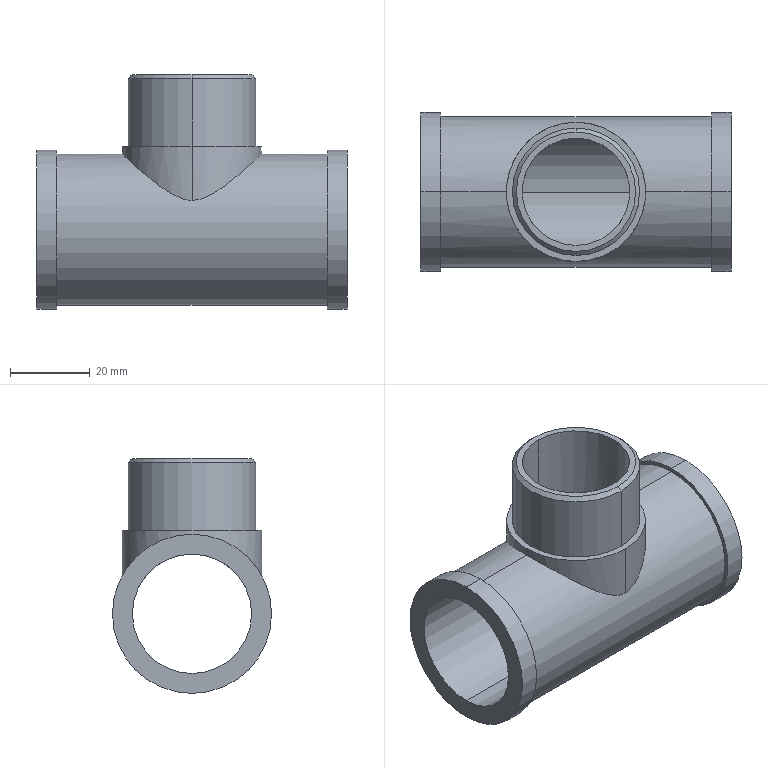Part | SolidWorks | features ICE 2, Revolution 2, Chamfer 1 | 1 solid | 22 faces | box 78 x 40 x 59 mm | volume 38405 mm3 | cylinder 14 | plane 6 | cone 2 | commonest cylinder face diameters 40 x4 27 x2 30 x2 32 x2 35 x2 38 x2
STEP:
#1=CARTESIAN_POINT('',(39.,-15.,39.));
#2=VERTEX_POINT('',#1);
#3=CARTESIAN_POINT('',(39.,15.,39.));
#4=VERTEX_POINT('',#3);
#5=CARTESIAN_POINT('',(39.,0.,39.));
#6=DIRECTION('',(0.,0.,1.));
#7=DIRECTION('',(0.,1.,0.));
#8=AXIS2_PLACEMENT_3D('',#5,#6,#7);
#9=CIRCLE('',#8,15.);
#10=EDGE_CURVE('',#2,#4,#9,.T.);
#11=ORIENTED_EDGE('',*,*,#10,.F.);
#12=CARTESIAN_POINT('',(39.,-16.,38.));
#13=VERTEX_POINT('',#12);
#14=CARTESIAN_POINT('',(39.,-16.,38.));
#15=DIRECTION('',(0.,-0.7071,-0.7071));
#16=VECTOR('',#15,1000.);
#17=LINE('',#14,#16);
#18=EDGE_CURVE('',#2,#13,#17,.T.);
#19=ORIENTED_EDGE('',*,*,#18,.T.);
#20=CARTESIAN_POINT('',(39.,16.,38.));
#21=VERTEX_POINT('',#20);
#22=CARTESIAN_POINT('',(39.,0.,38.));
#23=DIRECTION('',(0.,0.,-1.));
#24=DIRECTION('',(0.,1.,0.));
#25=AXIS2_PLACEMENT_3D('',#22,#23,#24);
#26=CIRCLE('',#25,16.);
#27=EDGE_CURVE('',#21,#13,#26,.T.);
#28=ORIENTED_EDGE('',*,*,#27,.F.);
#29=CARTESIAN_POINT('',(39.,16.,38.));
#30=DIRECTION('',(0.,0.7071,-0.7071));
#31=VECTOR('',#30,1000.);
#32=LINE('',#29,#31);
#33=EDGE_CURVE('',#4,#21,#32,.T.);
#34=ORIENTED_EDGE('',*,*,#33,.F.);
#35=EDGE_LOOP('',(#11,#19,#28,#34));
#36=FACE_OUTER_BOUND('',#35,.T.);
#37=CARTESIAN_POINT('',(39.,0.,38.));
#38=DIRECTION('',(0.,0.,-1.));
#39=DIRECTION('',(0.,1.,0.));
#40=AXIS2_PLACEMENT_3D('',#37,#38,#39);
#41=CONICAL_SURFACE('',#40,16.,0.7854);
#42=ADVANCED_FACE('',(#36),#41,.T.);
#43=CARTESIAN_POINT('',(78.,0.,-15.));
#44=VERTEX_POINT('',#43);
#45=CARTESIAN_POINT('',(78.,0.,15.));
#46=VERTEX_POINT('',#45);
#47=CARTESIAN_POINT('',(78.,0.,0.));
#48=DIRECTION('',(-1.,0.,0.));
#49=DIRECTION('',(0.,0.,1.));
#50=AXIS2_PLACEMENT_3D('',#47,#48,#49);
#51=CIRCLE('',#50,15.);
#52=EDGE_CURVE('',#44,#46,#51,.T.);
#53=ORIENTED_EDGE('',*,*,#52,.F.);
#54=CARTESIAN_POINT('',(0.,0.,-15.));
#55=VERTEX_POINT('',#54);
#56=CARTESIAN_POINT('',(0.,0.,-15.));
#57=DIRECTION('',(-1.,0.,0.));
#58=VECTOR('',#57,1000.);
#59=LINE('',#56,#58);
#60=EDGE_CURVE('',#44,#55,#59,.T.);
#61=ORIENTED_EDGE('',*,*,#60,.T.);
#62=CARTESIAN_POINT('',(0.,0.,15.));
#63=VERTEX_POINT('',#62);
#64=CARTESIAN_POINT('',(0.,0.,0.));
#65=DIRECTION('',(-1.,0.,0.));
#66=DIRECTION('',(0.,0.,1.));
#67=AXIS2_PLACEMENT_3D('',#64,#65,#66);
#68=CIRCLE('',#67,15.);
#69=EDGE_CURVE('',#55,#63,#68,.T.);
#70=ORIENTED_EDGE('',*,*,#69,.T.);
#71=CARTESIAN_POINT('',(25.5,0.,15.));
#72=VERTEX_POINT('',#71);
#73=CARTESIAN_POINT('',(0.,0.,15.));
#74=DIRECTION('',(-1.,0.,0.));
#75=VECTOR('',#74,1000.);
#76=LINE('',#73,#75);
#77=EDGE_CURVE('',#72,#63,#76,.T.);
#78=ORIENTED_EDGE('',*,*,#77,.F.);
#79=CARTESIAN_POINT('',(39.,-13.5,6.538));
#80=VERTEX_POINT('',#79);
#81=CARTESIAN_POINT('',(39.,-13.5,6.538));
#82=CARTESIAN_POINT('',(38.513,-13.5,6.538));
#83=CARTESIAN_POINT('',(38.035,-13.474,6.593));
#84=CARTESIAN_POINT('',(37.329,-13.398,6.745));
#85=CARTESIAN_POINT('',(37.094,-13.367,6.807));
#86=CARTESIAN_POINT('',(36.634,-13.293,6.95));
#87=CARTESIAN_POINT('',(36.41,-13.251,7.03));
#88=CARTESIAN_POINT('',(35.749,-13.11,7.291));
#89=CARTESIAN_POINT('',(35.325,-12.997,7.492));
#90=CARTESIAN_POINT('',(34.503,-12.736,7.928));
#91=CARTESIAN_POINT('',(34.103,-12.587,8.164));
#92=CARTESIAN_POINT('',(32.947,-12.096,8.89));
#93=CARTESIAN_POINT('',(32.232,-11.709,9.4));
#94=CARTESIAN_POINT('',(31.215,-11.037,10.164));
#95=CARTESIAN_POINT('',(30.885,-10.797,10.419));
#96=CARTESIAN_POINT('',(30.244,-10.284,10.926));
#97=CARTESIAN_POINT('',(29.931,-10.009,11.179));
#98=CARTESIAN_POINT('',(29.032,-9.142,11.916));
#99=CARTESIAN_POINT('',(28.482,-8.507,12.382));
#100=CARTESIAN_POINT('',(27.736,-7.454,13.024));
#101=CARTESIAN_POINT('',(27.5,-7.086,13.228));
#102=CARTESIAN_POINT('',(27.058,-6.312,13.614));
#103=CARTESIAN_POINT('',(26.853,-5.909,13.794));
#104=CARTESIAN_POINT('',(26.484,-5.081,14.12));
#105=CARTESIAN_POINT('',(26.319,-4.654,14.267));
#106=CARTESIAN_POINT('',(26.102,-3.992,14.461));
#107=CARTESIAN_POINT('',(26.034,-3.768,14.521));
#108=CARTESIAN_POINT('',(25.911,-3.313,14.632));
#109=CARTESIAN_POINT('',(25.854,-3.08,14.682));
#110=CARTESIAN_POINT('',(25.602,-1.914,14.908));
#111=CARTESIAN_POINT('',(25.5,-0.9652,15.));
#112=CARTESIAN_POINT('',(25.5,0.,15.));
#113=B_SPLINE_CURVE_WITH_KNOTS('',3,(#81,#82,#83,#84,#85,#86,#87,#88,#89,#90,#91,#92,#93,#94,#95,#96,#97,#98,#99,#100,#101,#102,#103,#104,#105,#106,#107,#108,#109,#110,#111,#112),.UNSPECIFIED.,.F.,.F.,(4,2,2,2,2,2,2,2,2,2,2,2,2,2,2,4),(0.02301,0.02446,0.02518,0.0259,0.02734,0.02879,0.03167,0.03311,0.03456,0.03744,0.03889,0.04033,0.04177,0.04249,0.04321,0.0461),.UNSPECIFIED.);
#114=EDGE_CURVE('',#80,#72,#113,.T.);
#115=ORIENTED_EDGE('',*,*,#114,.F.);
#116=CARTESIAN_POINT('',(52.5,0.,15.));
#117=VERTEX_POINT('',#116);
#118=CARTESIAN_POINT('',(52.5,0.,15.));
#119=CARTESIAN_POINT('',(52.5,-0.9754,15.));
#120=CARTESIAN_POINT('',(52.396,-1.925,14.906));
#121=CARTESIAN_POINT('',(52.096,-3.313,14.637));
#122=CARTESIAN_POINT('',(51.971,-3.773,14.525));
#123=CARTESIAN_POINT('',(51.679,-4.658,14.266));
#124=CARTESIAN_POINT('',(51.514,-5.086,14.119));
#125=CARTESIAN_POINT('',(51.145,-5.913,13.793));
#126=CARTESIAN_POINT('',(50.942,-6.312,13.614));
#127=CARTESIAN_POINT('',(50.5,-7.085,13.228));
#128=CARTESIAN_POINT('',(50.263,-7.456,13.022));
#129=CARTESIAN_POINT('',(49.515,-8.51,12.38));
#130=CARTESIAN_POINT('',(48.967,-9.143,11.915));
#131=CARTESIAN_POINT('',(48.072,-10.006,11.181));
#132=CARTESIAN_POINT('',(47.76,-10.28,10.929));
#133=CARTESIAN_POINT('',(47.117,-10.795,10.421));
#134=CARTESIAN_POINT('',(46.787,-11.035,10.165));
#135=CARTESIAN_POINT('',(45.768,-11.71,9.399));
#136=CARTESIAN_POINT('',(45.052,-12.096,8.889));
#137=CARTESIAN_POINT('',(43.898,-12.587,8.164));
#138=CARTESIAN_POINT('',(43.498,-12.736,7.928));
#139=CARTESIAN_POINT('',(42.675,-12.997,7.492));
#140=CARTESIAN_POINT('',(42.251,-13.111,7.291));
#141=CARTESIAN_POINT('',(41.367,-13.299,6.942));
#142=CARTESIAN_POINT('',(40.906,-13.373,6.795));
#143=CARTESIAN_POINT('',(40.204,-13.448,6.644));
#144=CARTESIAN_POINT('',(39.967,-13.467,6.605));
#145=CARTESIAN_POINT('',(39.487,-13.493,6.552));
#146=CARTESIAN_POINT('',(39.243,-13.5,6.538));
#147=CARTESIAN_POINT('',(39.,-13.5,6.538));
#148=B_SPLINE_CURVE_WITH_KNOTS('',3,(#118,#119,#120,#121,#122,#123,#124,#125,#126,#127,#128,#129,#130,#131,#132,#133,#134,#135,#136,#137,#138,#139,#140,#141,#142,#143,#144,#145,#146,#147),.UNSPECIFIED.,.F.,.F.,(4,2,2,2,2,2,2,2,2,2,2,2,2,2,4),(0.,0.002877,0.004315,0.005754,0.007192,0.008631,0.01151,0.01295,0.01438,0.01726,0.0187,0.02014,0.02158,0.0223,0.02301),.UNSPECIFIED.);
#149=EDGE_CURVE('',#117,#80,#148,.T.);
#150=ORIENTED_EDGE('',*,*,#149,.F.);
#151=CARTESIAN_POINT('',(0.,0.,15.));
#152=DIRECTION('',(-1.,0.,0.));
#153=VECTOR('',#152,1000.);
#154=LINE('',#151,#153);
#155=EDGE_CURVE('',#46,#117,#154,.T.);
#156=ORIENTED_EDGE('',*,*,#155,.F.);
#157=EDGE_LOOP('',(#53,#61,#70,#78,#115,#150,#156));
#158=FACE_OUTER_BOUND('',#157,.T.);
#159=CARTESIAN_POINT('',(0.,0.,0.));
#160=DIRECTION('',(-1.,0.,0.));
#161=DIRECTION('',(0.,0.,1.));
#162=AXIS2_PLACEMENT_3D('',#159,#160,#161);
#163=CYLINDRICAL_SURFACE('',#162,15.);
#164=ADVANCED_FACE('',(#158),#163,.F.);
#165=CARTESIAN_POINT('',(39.,17.5,21.));
#166=VERTEX_POINT('',#165);
#167=CARTESIAN_POINT('',(39.,-17.5,21.));
#168=VERTEX_POINT('',#167);
#169=CARTESIAN_POINT('',(39.,0.,21.));
#170=DIRECTION('',(0.,0.,-1.));
#171=DIRECTION('',(0.,1.,0.));
#172=AXIS2_PLACEMENT_3D('',#169,#170,#171);
#173=CIRCLE('',#172,17.5);
#174=EDGE_CURVE('',#166,#168,#173,.T.);
#175=ORIENTED_EDGE('',*,*,#174,.T.);
#176=CARTESIAN_POINT('',(39.,-17.5,7.399));
#177=VERTEX_POINT('',#176);
#178=CARTESIAN_POINT('',(39.,-17.5,0.));
#179=DIRECTION('',(0.,0.,-1.));
#180=VECTOR('',#179,1000.);
#181=LINE('',#178,#180);
#182=EDGE_CURVE('',#168,#177,#181,.T.);
#183=ORIENTED_EDGE('',*,*,#182,.T.);
#184=CARTESIAN_POINT('',(56.5,0.,19.));
#185=VERTEX_POINT('',#184);
#186=CARTESIAN_POINT('',(39.,-17.5,7.399));
#187=CARTESIAN_POINT('',(39.315,-17.5,7.399));
#188=CARTESIAN_POINT('',(39.63,-17.491,7.42));
#189=CARTESIAN_POINT('',(40.259,-17.457,7.499));
#190=CARTESIAN_POINT('',(40.574,-17.432,7.559));
#191=CARTESIAN_POINT('',(41.493,-17.333,7.785));
#192=CARTESIAN_POINT('',(42.078,-17.237,7.998));
#193=CARTESIAN_POINT('',(42.93,-17.055,8.375));
#194=CARTESIAN_POINT('',(43.211,-16.988,8.51));
#195=CARTESIAN_POINT('',(43.76,-16.843,8.795));
#196=CARTESIAN_POINT('',(44.028,-16.764,8.943));
#197=CARTESIAN_POINT('',(44.817,-16.514,9.402));
#198=CARTESIAN_POINT('',(45.322,-16.327,9.726));
#199=CARTESIAN_POINT('',(46.304,-15.912,10.391));
#200=CARTESIAN_POINT('',(46.781,-15.684,10.733));
#201=CARTESIAN_POINT('',(47.711,-15.187,11.425));
#202=CARTESIAN_POINT('',(48.166,-14.917,11.777));
#203=CARTESIAN_POINT('',(49.486,-14.05,12.823));
#204=CARTESIAN_POINT('',(50.31,-13.397,13.51));
#205=CARTESIAN_POINT('',(51.47,-12.29,14.499));
#206=CARTESIAN_POINT('',(51.843,-11.899,14.821));
#207=CARTESIAN_POINT('',(52.564,-11.071,15.45));
#208=CARTESIAN_POINT('',(52.91,-10.633,15.755));
#209=CARTESIAN_POINT('',(53.887,-9.267,16.622));
#210=CARTESIAN_POINT('',(54.463,-8.279,17.141));
#211=CARTESIAN_POINT('',(55.073,-6.928,17.694));
#212=CARTESIAN_POINT('',(55.19,-6.651,17.8));
#213=CARTESIAN_POINT('',(55.409,-6.09,18.));
#214=CARTESIAN_POINT('',(55.511,-5.807,18.093));
#215=CARTESIAN_POINT('',(55.798,-4.945,18.355));
#216=CARTESIAN_POINT('',(55.96,-4.357,18.504));
#217=CARTESIAN_POINT('',(56.159,-3.452,18.686));
#218=CARTESIAN_POINT('',(56.218,-3.147,18.74));
#219=CARTESIAN_POINT('',(56.319,-2.529,18.834));
#220=CARTESIAN_POINT('',(56.362,-2.215,18.873));
#221=CARTESIAN_POINT('',(56.431,-1.585,18.936));
#222=CARTESIAN_POINT('',(56.457,-1.27,18.96));
#223=CARTESIAN_POINT('',(56.491,-0.6365,18.992));
#224=CARTESIAN_POINT('',(56.5,-0.3201,19.));
#225=CARTESIAN_POINT('',(56.5,0.,19.));
#226=B_SPLINE_CURVE_WITH_KNOTS('',3,(#186,#187,#188,#189,#190,#191,#192,#193,#194,#195,#196,#197,#198,#199,#200,#201,#202,#203,#204,#205,#206,#207,#208,#209,#210,#211,#212,#213,#214,#215,#216,#217,#218,#219,#220,#221,#222,#223,#224,#225),.UNSPECIFIED.,.F.,.F.,(4,2,2,2,2,2,2,2,2,2,2,2,2,2,2,2,2,2,2,4),(0.09049,0.09144,0.09238,0.09427,0.09521,0.09616,0.09805,0.09993,0.1018,0.1056,0.1075,0.1094,0.1132,0.1141,0.115,0.1169,0.1179,0.1188,0.1198,0.1207),.UNSPECIFIED.);
#227=EDGE_CURVE('',#177,#185,#226,.T.);
#228=ORIENTED_EDGE('',*,*,#227,.T.);
#229=CARTESIAN_POINT('',(39.,17.5,7.399));
#230=VERTEX_POINT('',#229);
#231=CARTESIAN_POINT('',(56.5,0.,19.));
#232=CARTESIAN_POINT('',(56.5,1.276,19.));
#233=CARTESIAN_POINT('',(56.362,2.518,18.873));
#234=CARTESIAN_POINT('',(55.967,4.332,18.51));
#235=CARTESIAN_POINT('',(55.801,4.933,18.358));
#236=CARTESIAN_POINT('',(55.419,6.087,18.009));
#237=CARTESIAN_POINT('',(55.201,6.643,17.81));
#238=CARTESIAN_POINT('',(54.716,7.72,17.371));
#239=CARTESIAN_POINT('',(54.45,8.239,17.13));
#240=CARTESIAN_POINT('',(53.871,9.244,16.609));
#241=CARTESIAN_POINT('',(53.561,9.723,16.333));
#242=CARTESIAN_POINT('',(52.586,11.087,15.468));
#243=CARTESIAN_POINT('',(51.871,11.905,14.841));
#244=CARTESIAN_POINT('',(50.708,13.018,13.849));
#245=CARTESIAN_POINT('',(50.303,13.37,13.508));
#246=CARTESIAN_POINT('',(49.472,14.031,12.82));
#247=CARTESIAN_POINT('',(49.046,14.339,12.474));
#248=CARTESIAN_POINT('',(47.731,15.203,11.432));
#249=CARTESIAN_POINT('',(46.809,15.698,10.733));
#250=CARTESIAN_POINT('',(45.326,16.325,9.728));
#251=CARTESIAN_POINT('',(44.814,16.515,9.401));
#252=CARTESIAN_POINT('',(43.76,16.849,8.788));
#253=CARTESIAN_POINT('',(43.215,16.995,8.5));
#254=CARTESIAN_POINT('',(42.074,17.238,7.996));
#255=CARTESIAN_POINT('',(41.485,17.333,7.783));
#256=CARTESIAN_POINT('',(40.573,17.432,7.559));
#257=CARTESIAN_POINT('',(40.263,17.457,7.5));
#258=CARTESIAN_POINT('',(39.632,17.491,7.42));
#259=CARTESIAN_POINT('',(39.314,17.5,7.399));
#260=CARTESIAN_POINT('',(39.,17.5,7.399));
#261=B_SPLINE_CURVE_WITH_KNOTS('',3,(#231,#232,#233,#234,#235,#236,#237,#238,#239,#240,#241,#242,#243,#244,#245,#246,#247,#248,#249,#250,#251,#252,#253,#254,#255,#256,#257,#258,#259,#260),.UNSPECIFIED.,.F.,.F.,(4,2,2,2,2,2,2,2,2,2,2,2,2,2,4),(0.,0.003764,0.005646,0.007528,0.00941,0.01129,0.01506,0.01694,0.01882,0.02258,0.02447,0.02635,0.02823,0.02917,0.03011),.UNSPECIFIED.);
#262=EDGE_CURVE('',#185,#230,#261,.T.);
#263=ORIENTED_EDGE('',*,*,#262,.T.);
#264=CARTESIAN_POINT('',(39.,17.5,0.));
#265=DIRECTION('',(0.,0.,-1.));
#266=VECTOR('',#265,1000.);
#267=LINE('',#264,#266);
#268=EDGE_CURVE('',#166,#230,#267,.T.);
#269=ORIENTED_EDGE('',*,*,#268,.F.);
#270=EDGE_LOOP('',(#175,#183,#228,#263,#269));
#271=FACE_OUTER_BOUND('',#270,.T.);
#272=CARTESIAN_POINT('',(39.,0.,0.));
#273=DIRECTION('',(0.,0.,-1.));
#274=DIRECTION('',(0.,1.,0.));
#275=AXIS2_PLACEMENT_3D('',#272,#273,#274);
#276=CYLINDRICAL_SURFACE('',#275,17.5);
#277=ADVANCED_FACE('',(#271),#276,.T.);
#278=CARTESIAN_POINT('',(39.,-13.5,39.));
#279=VERTEX_POINT('',#278);
#280=CARTESIAN_POINT('',(39.,13.5,39.));
#281=VERTEX_POINT('',#280);
#282=CARTESIAN_POINT('',(39.,0.,39.));
#283=DIRECTION('',(0.,0.,-1.));
#284=DIRECTION('',(0.,1.,0.));
#285=AXIS2_PLACEMENT_3D('',#282,#283,#284);
#286=CIRCLE('',#285,13.5);
#287=EDGE_CURVE('',#279,#281,#286,.T.);
#288=ORIENTED_EDGE('',*,*,#287,.F.);
#289=CARTESIAN_POINT('',(39.,-13.5,0.));
#290=DIRECTION('',(0.,0.,-1.));
#291=VECTOR('',#290,1000.);
#292=LINE('',#289,#291);
#293=EDGE_CURVE('',#279,#80,#292,.T.);
#294=ORIENTED_EDGE('',*,*,#293,.T.);
#295=ORIENTED_EDGE('',*,*,#114,.T.);
#296=CARTESIAN_POINT('',(39.,13.5,6.538));
#297=VERTEX_POINT('',#296);
#298=CARTESIAN_POINT('',(25.5,0.,15.));
#299=CARTESIAN_POINT('',(25.5,0.4816,15.));
#300=CARTESIAN_POINT('',(25.526,0.9708,14.976));
#301=CARTESIAN_POINT('',(25.63,1.926,14.884));
#302=CARTESIAN_POINT('',(25.706,2.396,14.815));
#303=CARTESIAN_POINT('',(25.906,3.32,14.636));
#304=CARTESIAN_POINT('',(26.03,3.775,14.525));
#305=CARTESIAN_POINT('',(26.323,4.665,14.264));
#306=CARTESIAN_POINT('',(26.489,5.093,14.116));
#307=CARTESIAN_POINT('',(26.859,5.92,13.789));
#308=CARTESIAN_POINT('',(27.062,6.319,13.611));
#309=CARTESIAN_POINT('',(27.503,7.09,13.225));
#310=CARTESIAN_POINT('',(27.741,7.462,13.019));
#311=CARTESIAN_POINT('',(28.49,8.517,12.375));
#312=CARTESIAN_POINT('',(29.039,9.149,11.91));
#313=CARTESIAN_POINT('',(30.231,10.297,10.933));
#314=CARTESIAN_POINT('',(30.877,10.814,10.417));
#315=CARTESIAN_POINT('',(32.237,11.712,9.396));
#316=CARTESIAN_POINT('',(32.952,12.098,8.886));
#317=CARTESIAN_POINT('',(34.103,12.588,8.163));
#318=CARTESIAN_POINT('',(34.502,12.736,7.928));
#319=CARTESIAN_POINT('',(35.327,12.998,7.491));
#320=CARTESIAN_POINT('',(35.751,13.111,7.29));
#321=CARTESIAN_POINT('',(36.633,13.299,6.942));
#322=CARTESIAN_POINT('',(37.096,13.373,6.795));
#323=CARTESIAN_POINT('',(38.034,13.474,6.593));
#324=CARTESIAN_POINT('',(38.512,13.5,6.538));
#325=CARTESIAN_POINT('',(39.,13.5,6.538));
#326=B_SPLINE_CURVE_WITH_KNOTS('',3,(#298,#299,#300,#301,#302,#303,#304,#305,#306,#307,#308,#309,#310,#311,#312,#313,#314,#315,#316,#317,#318,#319,#320,#321,#322,#323,#324,#325),.UNSPECIFIED.,.F.,.F.,(4,2,2,2,2,2,2,2,2,2,2,2,2,4),(0.0461,0.04754,0.04898,0.05042,0.05186,0.0533,0.05474,0.05762,0.0605,0.06338,0.06482,0.06626,0.0677,0.06914),.UNSPECIFIED.);
#327=EDGE_CURVE('',#72,#297,#326,.T.);
#328=ORIENTED_EDGE('',*,*,#327,.T.);
#329=CARTESIAN_POINT('',(39.,13.5,0.));
#330=DIRECTION('',(0.,0.,-1.));
#331=VECTOR('',#330,1000.);
#332=LINE('',#329,#331);
#333=EDGE_CURVE('',#281,#297,#332,.T.);
#334=ORIENTED_EDGE('',*,*,#333,.F.);
#335=EDGE_LOOP('',(#288,#294,#295,#328,#334));
#336=FACE_OUTER_BOUND('',#335,.T.);
#337=CARTESIAN_POINT('',(39.,0.,0.));
#338=DIRECTION('',(0.,0.,-1.));
#339=DIRECTION('',(0.,1.,0.));
#340=AXIS2_PLACEMENT_3D('',#337,#338,#339);
#341=CYLINDRICAL_SURFACE('',#340,13.5);
#342=ADVANCED_FACE('',(#336),#341,.F.);
#343=ORIENTED_EDGE('',*,*,#27,.T.);
#344=CARTESIAN_POINT('',(39.,-16.,21.));
#345=VERTEX_POINT('',#344);
#346=CARTESIAN_POINT('',(39.,-16.,0.));
#347=DIRECTION('',(0.,0.,-1.));
#348=VECTOR('',#347,1000.);
#349=LINE('',#346,#348);
#350=EDGE_CURVE('',#13,#345,#349,.T.);
#351=ORIENTED_EDGE('',*,*,#350,.T.);
#352=CARTESIAN_POINT('',(39.,16.,21.));
#353=VERTEX_POINT('',#352);
#354=CARTESIAN_POINT('',(39.,0.,21.));
#355=DIRECTION('',(0.,0.,-1.));
#356=DIRECTION('',(0.,1.,0.));
#357=AXIS2_PLACEMENT_3D('',#354,#355,#356);
#358=CIRCLE('',#357,16.);
#359=EDGE_CURVE('',#353,#345,#358,.T.);
#360=ORIENTED_EDGE('',*,*,#359,.F.);
#361=CARTESIAN_POINT('',(39.,16.,0.));
#362=DIRECTION('',(0.,0.,-1.));
#363=VECTOR('',#362,1000.);
#364=LINE('',#361,#363);
#365=EDGE_CURVE('',#21,#353,#364,.T.);
#366=ORIENTED_EDGE('',*,*,#365,.F.);
#367=EDGE_LOOP('',(#343,#351,#360,#366));
#368=FACE_OUTER_BOUND('',#367,.T.);
#369=CARTESIAN_POINT('',(39.,0.,0.));
#370=DIRECTION('',(0.,0.,-1.));
#371=DIRECTION('',(0.,1.,0.));
#372=AXIS2_PLACEMENT_3D('',#369,#370,#371);
#373=CYLINDRICAL_SURFACE('',#372,16.);
#374=ADVANCED_FACE('',(#368),#373,.T.);
#375=CARTESIAN_POINT('',(78.,0.,20.));
#376=VERTEX_POINT('',#375);
#377=CARTESIAN_POINT('',(78.,0.,-20.));
#378=VERTEX_POINT('',#377);
#379=CARTESIAN_POINT('',(78.,0.,0.));
#380=DIRECTION('',(-1.,0.,0.));
#381=DIRECTION('',(0.,0.,1.));
#382=AXIS2_PLACEMENT_3D('',#379,#380,#381);
#383=CIRCLE('',#382,20.);
#384=EDGE_CURVE('',#376,#378,#383,.T.);
#385=ORIENTED_EDGE('',*,*,#384,.T.);
#386=CARTESIAN_POINT('',(73.,0.,-20.));
#387=VERTEX_POINT('',#386);
#388=CARTESIAN_POINT('',(0.,0.,-20.));
#389=DIRECTION('',(-1.,0.,0.));
#390=VECTOR('',#389,1000.);
#391=LINE('',#388,#390);
#392=EDGE_CURVE('',#378,#387,#391,.T.);
#393=ORIENTED_EDGE('',*,*,#392,.T.);
#394=CARTESIAN_POINT('',(73.,0.,20.));
#395=VERTEX_POINT('',#394);
#396=CARTESIAN_POINT('',(73.,0.,0.));
#397=DIRECTION('',(-1.,0.,0.));
#398=DIRECTION('',(0.,0.,1.));
#399=AXIS2_PLACEMENT_3D('',#396,#397,#398);
#400=CIRCLE('',#399,20.);
#401=EDGE_CURVE('',#395,#387,#400,.T.);
#402=ORIENTED_EDGE('',*,*,#401,.F.);
#403=CARTESIAN_POINT('',(0.,0.,20.));
#404=DIRECTION('',(-1.,0.,0.));
#405=VECTOR('',#404,1000.);
#406=LINE('',#403,#405);
#407=EDGE_CURVE('',#376,#395,#406,.T.);
#408=ORIENTED_EDGE('',*,*,#407,.F.);
#409=EDGE_LOOP('',(#385,#393,#402,#408));
#410=FACE_OUTER_BOUND('',#409,.T.);
#411=CARTESIAN_POINT('',(0.,0.,0.));
#412=DIRECTION('',(-1.,0.,0.));
#413=DIRECTION('',(0.,0.,1.));
#414=AXIS2_PLACEMENT_3D('',#411,#412,#413);
#415=CYLINDRICAL_SURFACE('',#414,20.);
#416=ADVANCED_FACE('',(#410),#415,.T.);
#417=CARTESIAN_POINT('',(5.,0.,20.));
#418=VERTEX_POINT('',#417);
#419=CARTESIAN_POINT('',(5.,0.,-20.));
#420=VERTEX_POINT('',#419);
#421=CARTESIAN_POINT('',(5.,0.,0.));
#422=DIRECTION('',(-1.,0.,0.));
#423=DIRECTION('',(0.,0.,1.));
#424=AXIS2_PLACEMENT_3D('',#421,#422,#423);
#425=CIRCLE('',#424,20.);
#426=EDGE_CURVE('',#418,#420,#425,.T.);
#427=ORIENTED_EDGE('',*,*,#426,.T.);
#428=CARTESIAN_POINT('',(0.,0.,-20.));
#429=VERTEX_POINT('',#428);
#430=CARTESIAN_POINT('',(0.,0.,-20.));
#431=DIRECTION('',(-1.,0.,0.));
#432=VECTOR('',#431,1000.);
#433=LINE('',#430,#432);
#434=EDGE_CURVE('',#420,#429,#433,.T.);
#435=ORIENTED_EDGE('',*,*,#434,.T.);
#436=CARTESIAN_POINT('',(0.,0.,20.));
#437=VERTEX_POINT('',#436);
#438=CARTESIAN_POINT('',(0.,0.,0.));
#439=DIRECTION('',(-1.,0.,0.));
#440=DIRECTION('',(0.,0.,1.));
#441=AXIS2_PLACEMENT_3D('',#438,#439,#440);
#442=CIRCLE('',#441,20.);
#443=EDGE_CURVE('',#437,#429,#442,.T.);
#444=ORIENTED_EDGE('',*,*,#443,.F.);
#445=CARTESIAN_POINT('',(0.,0.,20.));
#446=DIRECTION('',(-1.,0.,0.));
#447=VECTOR('',#446,1000.);
#448=LINE('',#445,#447);
#449=EDGE_CURVE('',#418,#437,#448,.T.);
#450=ORIENTED_EDGE('',*,*,#449,.F.);
#451=EDGE_LOOP('',(#427,#435,#444,#450));
#452=FACE_OUTER_BOUND('',#451,.T.);
#453=CARTESIAN_POINT('',(0.,0.,0.));
#454=DIRECTION('',(-1.,0.,0.));
#455=DIRECTION('',(0.,0.,1.));
#456=AXIS2_PLACEMENT_3D('',#453,#454,#455);
#457=CYLINDRICAL_SURFACE('',#456,20.);
#458=ADVANCED_FACE('',(#452),#457,.T.);
#459=CARTESIAN_POINT('',(73.,0.,19.));
#460=VERTEX_POINT('',#459);
#461=CARTESIAN_POINT('',(73.,0.,-19.));
#462=VERTEX_POINT('',#461);
#463=CARTESIAN_POINT('',(73.,0.,0.));
#464=DIRECTION('',(-1.,0.,0.));
#465=DIRECTION('',(0.,0.,1.));
#466=AXIS2_PLACEMENT_3D('',#463,#464,#465);
#467=CIRCLE('',#466,19.);
#468=EDGE_CURVE('',#460,#462,#467,.T.);
#469=ORIENTED_EDGE('',*,*,#468,.T.);
#470=CARTESIAN_POINT('',(5.,0.,-19.));
#471=VERTEX_POINT('',#470);
#472=CARTESIAN_POINT('',(0.,0.,-19.));
#473=DIRECTION('',(-1.,0.,0.));
#474=VECTOR('',#473,1000.);
#475=LINE('',#472,#474);
#476=EDGE_CURVE('',#462,#471,#475,.T.);
#477=ORIENTED_EDGE('',*,*,#476,.T.);
#478=CARTESIAN_POINT('',(5.,0.,19.));
#479=VERTEX_POINT('',#478);
#480=CARTESIAN_POINT('',(5.,0.,0.));
#481=DIRECTION('',(-1.,0.,0.));
#482=DIRECTION('',(0.,0.,1.));
#483=AXIS2_PLACEMENT_3D('',#480,#481,#482);
#484=CIRCLE('',#483,19.);
#485=EDGE_CURVE('',#479,#471,#484,.T.);
#486=ORIENTED_EDGE('',*,*,#485,.F.);
#487=CARTESIAN_POINT('',(21.5,0.,19.));
#488=VERTEX_POINT('',#487);
#489=CARTESIAN_POINT('',(0.,0.,19.));
#490=DIRECTION('',(-1.,0.,0.));
#491=VECTOR('',#490,1000.);
#492=LINE('',#489,#491);
#493=EDGE_CURVE('',#488,#479,#492,.T.);
#494=ORIENTED_EDGE('',*,*,#493,.F.);
#495=CARTESIAN_POINT('',(39.,17.5,7.399));
#496=CARTESIAN_POINT('',(38.369,17.5,7.399));
#497=CARTESIAN_POINT('',(37.746,17.466,7.481));
#498=CARTESIAN_POINT('',(36.82,17.366,7.708));
#499=CARTESIAN_POINT('',(36.517,17.325,7.8));
#500=CARTESIAN_POINT('',(35.926,17.23,8.008));
#501=CARTESIAN_POINT('',(35.637,17.176,8.124));
#502=CARTESIAN_POINT('',(34.787,16.995,8.5));
#503=CARTESIAN_POINT('',(34.24,16.849,8.788));
#504=CARTESIAN_POINT('',(33.179,16.513,9.405));
#505=CARTESIAN_POINT('',(32.671,16.324,9.73));
#506=CARTESIAN_POINT('',(31.195,15.7,10.73));
#507=CARTESIAN_POINT('',(30.274,15.206,11.428));
#508=CARTESIAN_POINT('',(28.954,14.339,12.474));
#509=CARTESIAN_POINT('',(28.524,14.028,12.824));
#510=CARTESIAN_POINT('',(27.692,13.366,13.512));
#511=CARTESIAN_POINT('',(27.291,13.017,13.849));
#512=CARTESIAN_POINT('',(26.133,11.91,14.837));
#513=CARTESIAN_POINT('',(25.42,11.094,15.462));
#514=CARTESIAN_POINT('',(24.444,9.73,16.328));
#515=CARTESIAN_POINT('',(24.133,9.25,16.606));
#516=CARTESIAN_POINT('',(23.553,8.245,17.127));
#517=CARTESIAN_POINT('',(23.286,7.724,17.369));
#518=CARTESIAN_POINT('',(22.801,6.647,17.809));
#519=CARTESIAN_POINT('',(22.583,6.09,18.008));
#520=CARTESIAN_POINT('',(22.199,4.935,18.358));
#521=CARTESIAN_POINT('',(22.034,4.333,18.51));
#522=CARTESIAN_POINT('',(21.637,2.513,18.874));
#523=CARTESIAN_POINT('',(21.5,1.272,19.));
#524=CARTESIAN_POINT('',(21.5,0.,19.));
#525=B_SPLINE_CURVE_WITH_KNOTS('',3,(#495,#496,#497,#498,#499,#500,#501,#502,#503,#504,#505,#506,#507,#508,#509,#510,#511,#512,#513,#514,#515,#516,#517,#518,#519,#520,#521,#522,#523,#524),.UNSPECIFIED.,.F.,.F.,(4,2,2,2,2,2,2,2,2,2,2,2,2,2,4),(0.03011,0.032,0.03295,0.03389,0.03578,0.03767,0.04145,0.04334,0.04523,0.04901,0.0509,0.05279,0.05468,0.05657,0.06035),.UNSPECIFIED.);
#526=EDGE_CURVE('',#230,#488,#525,.T.);
#527=ORIENTED_EDGE('',*,*,#526,.F.);
#528=ORIENTED_EDGE('',*,*,#262,.F.);
#529=CARTESIAN_POINT('',(0.,0.,19.));
#530=DIRECTION('',(-1.,0.,0.));
#531=VECTOR('',#530,1000.);
#532=LINE('',#529,#531);
#533=EDGE_CURVE('',#460,#185,#532,.T.);
#534=ORIENTED_EDGE('',*,*,#533,.F.);
#535=EDGE_LOOP('',(#469,#477,#486,#494,#527,#528,#534));
#536=FACE_OUTER_BOUND('',#535,.T.);
#537=CARTESIAN_POINT('',(0.,0.,0.));
#538=DIRECTION('',(-1.,0.,0.));
#539=DIRECTION('',(0.,0.,1.));
#540=AXIS2_PLACEMENT_3D('',#537,#538,#539);
#541=CYLINDRICAL_SURFACE('',#540,19.);
#542=ADVANCED_FACE('',(#536),#541,.T.);
#543=ORIENTED_EDGE('',*,*,#476,.F.);
#544=CARTESIAN_POINT('',(73.,0.,0.));
#545=DIRECTION('',(-1.,0.,0.));
#546=DIRECTION('',(0.,0.,1.));
#547=AXIS2_PLACEMENT_3D('',#544,#545,#546);
#548=CIRCLE('',#547,19.);
#549=EDGE_CURVE('',#462,#460,#548,.T.);
#550=ORIENTED_EDGE('',*,*,#549,.T.);
#551=ORIENTED_EDGE('',*,*,#533,.T.);
#552=ORIENTED_EDGE('',*,*,#227,.F.);
#553=CARTESIAN_POINT('',(21.5,0.,19.));
#554=CARTESIAN_POINT('',(21.5,-0.3169,19.));
#555=CARTESIAN_POINT('',(21.509,-0.6365,18.992));
#556=CARTESIAN_POINT('',(21.543,-1.269,18.96));
#557=CARTESIAN_POINT('',(21.569,-1.582,18.937));
#558=CARTESIAN_POINT('',(21.671,-2.516,18.843));
#559=CARTESIAN_POINT('',(21.771,-3.13,18.751));
#560=CARTESIAN_POINT('',(22.035,-4.339,18.508));
#561=CARTESIAN_POINT('',(22.2,-4.938,18.357));
#562=CARTESIAN_POINT('',(22.584,-6.093,18.007));
#563=CARTESIAN_POINT('',(22.802,-6.65,17.808));
#564=CARTESIAN_POINT('',(23.287,-7.727,17.368));
#565=CARTESIAN_POINT('',(23.554,-8.248,17.126));
#566=CARTESIAN_POINT('',(24.134,-9.252,16.605));
#567=CARTESIAN_POINT('',(24.442,-9.728,16.33));
#568=CARTESIAN_POINT('',(25.416,-11.09,15.465));
#569=CARTESIAN_POINT('',(26.131,-11.908,14.839));
#570=CARTESIAN_POINT('',(27.296,-13.021,13.845));
#571=CARTESIAN_POINT('',(27.701,-13.374,13.504));
#572=CARTESIAN_POINT('',(28.531,-14.033,12.818));
#573=CARTESIAN_POINT('',(28.957,-14.341,12.472));
#574=CARTESIAN_POINT('',(30.271,-15.204,11.431));
#575=CARTESIAN_POINT('',(31.193,-15.699,10.732));
#576=CARTESIAN_POINT('',(32.679,-16.327,9.725));
#577=CARTESIAN_POINT('',(33.188,-16.516,9.399));
#578=CARTESIAN_POINT('',(34.242,-16.85,8.787));
#579=CARTESIAN_POINT('',(34.788,-16.996,8.499));
#580=CARTESIAN_POINT('',(35.928,-17.238,7.995));
#581=CARTESIAN_POINT('',(36.514,-17.333,7.783));
#582=CARTESIAN_POINT('',(37.427,-17.432,7.559));
#583=CARTESIAN_POINT('',(37.738,-17.457,7.5));
#584=CARTESIAN_POINT('',(38.37,-17.492,7.419));
#585=CARTESIAN_POINT('',(38.685,-17.5,7.399));
#586=CARTESIAN_POINT('',(39.,-17.5,7.399));
#587=B_SPLINE_CURVE_WITH_KNOTS('',3,(#553,#554,#555,#556,#557,#558,#559,#560,#561,#562,#563,#564,#565,#566,#567,#568,#569,#570,#571,#572,#573,#574,#575,#576,#577,#578,#579,#580,#581,#582,#583,#584,#585,#586),.UNSPECIFIED.,.F.,.F.,(4,2,2,2,2,2,2,2,2,2,2,2,2,2,2,2,4),(0.06035,0.0613,0.06224,0.06412,0.06601,0.06789,0.06977,0.07166,0.07542,0.07731,0.07919,0.08296,0.08484,0.08673,0.08861,0.08955,0.09049),.UNSPECIFIED.);
#588=EDGE_CURVE('',#488,#177,#587,.T.);
#589=ORIENTED_EDGE('',*,*,#588,.F.);
#590=ORIENTED_EDGE('',*,*,#493,.T.);
#591=CARTESIAN_POINT('',(5.,0.,0.));
#592=DIRECTION('',(-1.,0.,0.));
#593=DIRECTION('',(0.,0.,1.));
#594=AXIS2_PLACEMENT_3D('',#591,#592,#593);
#595=CIRCLE('',#594,19.);
#596=EDGE_CURVE('',#471,#479,#595,.T.);
#597=ORIENTED_EDGE('',*,*,#596,.F.);
#598=EDGE_LOOP('',(#543,#550,#551,#552,#589,#590,#597));
#599=FACE_OUTER_BOUND('',#598,.T.);
#600=CARTESIAN_POINT('',(0.,0.,0.));
#601=DIRECTION('',(-1.,0.,0.));
#602=DIRECTION('',(0.,0.,1.));
#603=AXIS2_PLACEMENT_3D('',#600,#601,#602);
#604=CYLINDRICAL_SURFACE('',#603,19.);
#605=ADVANCED_FACE('',(#599),#604,.T.);
#606=ORIENTED_EDGE('',*,*,#434,.F.);
#607=CARTESIAN_POINT('',(5.,0.,0.));
#608=DIRECTION('',(-1.,0.,0.));
#609=DIRECTION('',(0.,0.,1.));
#610=AXIS2_PLACEMENT_3D('',#607,#608,#609);
#611=CIRCLE('',#610,20.);
#612=EDGE_CURVE('',#420,#418,#611,.T.);
#613=ORIENTED_EDGE('',*,*,#612,.T.);
#614=ORIENTED_EDGE('',*,*,#449,.T.);
#615=CARTESIAN_POINT('',(0.,0.,0.));
#616=DIRECTION('',(-1.,0.,0.));
#617=DIRECTION('',(0.,0.,1.));
#618=AXIS2_PLACEMENT_3D('',#615,#616,#617);
#619=CIRCLE('',#618,20.);
#620=EDGE_CURVE('',#429,#437,#619,.T.);
#621=ORIENTED_EDGE('',*,*,#620,.F.);
#622=EDGE_LOOP('',(#606,#613,#614,#621));
#623=FACE_OUTER_BOUND('',#622,.T.);
#624=CARTESIAN_POINT('',(0.,0.,0.));
#625=DIRECTION('',(-1.,0.,0.));
#626=DIRECTION('',(0.,0.,1.));
#627=AXIS2_PLACEMENT_3D('',#624,#625,#626);
#628=CYLINDRICAL_SURFACE('',#627,20.);
#629=ADVANCED_FACE('',(#623),#628,.T.);
#630=CARTESIAN_POINT('',(0.,0.,0.));
#631=DIRECTION('',(-1.,0.,0.));
#632=DIRECTION('',(0.,0.,1.));
#633=AXIS2_PLACEMENT_3D('',#630,#631,#632);
#634=CIRCLE('',#633,15.);
#635=EDGE_CURVE('',#63,#55,#634,.T.);
#636=ORIENTED_EDGE('',*,*,#635,.F.);
#637=ORIENTED_EDGE('',*,*,#69,.F.);
#638=EDGE_LOOP('',(#636,#637));
#639=FACE_BOUND('',#638,.T.);
#640=ORIENTED_EDGE('',*,*,#443,.T.);
#641=ORIENTED_EDGE('',*,*,#620,.T.);
#642=EDGE_LOOP('',(#640,#641));
#643=FACE_OUTER_BOUND('',#642,.T.);
#644=CARTESIAN_POINT('',(0.,20.,0.));
#645=DIRECTION('',(1.,0.,0.));
#646=DIRECTION('',(0.,0.,-1.));
#647=AXIS2_PLACEMENT_3D('',#644,#645,#646);
#648=PLANE('',#647);
#649=ADVANCED_FACE('',(#639,#643),#648,.F.);
#650=ORIENTED_EDGE('',*,*,#384,.F.);
#651=CARTESIAN_POINT('',(78.,0.,0.));
#652=DIRECTION('',(-1.,0.,0.));
#653=DIRECTION('',(0.,0.,1.));
#654=AXIS2_PLACEMENT_3D('',#651,#652,#653);
#655=CIRCLE('',#654,20.);
#656=EDGE_CURVE('',#378,#376,#655,.T.);
#657=ORIENTED_EDGE('',*,*,#656,.F.);
#658=EDGE_LOOP('',(#650,#657));
#659=FACE_OUTER_BOUND('',#658,.T.);
#660=CARTESIAN_POINT('',(78.,0.,0.));
#661=DIRECTION('',(-1.,0.,0.));
#662=DIRECTION('',(0.,0.,1.));
#663=AXIS2_PLACEMENT_3D('',#660,#661,#662);
#664=CIRCLE('',#663,15.);
#665=EDGE_CURVE('',#46,#44,#664,.T.);
#666=ORIENTED_EDGE('',*,*,#665,.T.);
#667=ORIENTED_EDGE('',*,*,#52,.T.);
#668=EDGE_LOOP('',(#666,#667));
#669=FACE_BOUND('',#668,.T.);
#670=CARTESIAN_POINT('',(78.,20.,0.));
#671=DIRECTION('',(-1.,0.,0.));
#672=DIRECTION('',(0.,0.,1.));
#673=AXIS2_PLACEMENT_3D('',#670,#671,#672);
#674=PLANE('',#673);
#675=ADVANCED_FACE('',(#659,#669),#674,.F.);
#676=ORIENTED_EDGE('',*,*,#392,.F.);
#677=ORIENTED_EDGE('',*,*,#656,.T.);
#678=ORIENTED_EDGE('',*,*,#407,.T.);
#679=CARTESIAN_POINT('',(73.,0.,0.));
#680=DIRECTION('',(-1.,0.,0.));
#681=DIRECTION('',(0.,0.,1.));
#682=AXIS2_PLACEMENT_3D('',#679,#680,#681);
#683=CIRCLE('',#682,20.);
#684=EDGE_CURVE('',#387,#395,#683,.T.);
#685=ORIENTED_EDGE('',*,*,#684,.F.);
#686=EDGE_LOOP('',(#676,#677,#678,#685));
#687=FACE_OUTER_BOUND('',#686,.T.);
#688=CARTESIAN_POINT('',(0.,0.,0.));
#689=DIRECTION('',(-1.,0.,0.));
#690=DIRECTION('',(0.,0.,1.));
#691=AXIS2_PLACEMENT_3D('',#688,#689,#690);
#692=CYLINDRICAL_SURFACE('',#691,20.);
#693=ADVANCED_FACE('',(#687),#692,.T.);
#694=ORIENTED_EDGE('',*,*,#468,.F.);
#695=ORIENTED_EDGE('',*,*,#549,.F.);
#696=EDGE_LOOP('',(#694,#695));
#697=FACE_BOUND('',#696,.T.);
#698=ORIENTED_EDGE('',*,*,#401,.T.);
#699=ORIENTED_EDGE('',*,*,#684,.T.);
#700=EDGE_LOOP('',(#698,#699));
#701=FACE_OUTER_BOUND('',#700,.T.);
#702=CARTESIAN_POINT('',(73.,20.,0.));
#703=DIRECTION('',(1.,0.,0.));
#704=DIRECTION('',(0.,0.,-1.));
#705=AXIS2_PLACEMENT_3D('',#702,#703,#704);
#706=PLANE('',#705);
#707=ADVANCED_FACE('',(#697,#701),#706,.F.);
#708=ORIENTED_EDGE('',*,*,#426,.F.);
#709=ORIENTED_EDGE('',*,*,#612,.F.);
#710=EDGE_LOOP('',(#708,#709));
#711=FACE_OUTER_BOUND('',#710,.T.);
#712=ORIENTED_EDGE('',*,*,#485,.T.);
#713=ORIENTED_EDGE('',*,*,#596,.T.);
#714=EDGE_LOOP('',(#712,#713));
#715=FACE_BOUND('',#714,.T.);
#716=CARTESIAN_POINT('',(5.,19.,0.));
#717=DIRECTION('',(-1.,0.,0.));
#718=DIRECTION('',(0.,0.,1.));
#719=AXIS2_PLACEMENT_3D('',#716,#717,#718);
#720=PLANE('',#719);
#721=ADVANCED_FACE('',(#711,#715),#720,.F.);
#722=ORIENTED_EDGE('',*,*,#350,.F.);
#723=CARTESIAN_POINT('',(39.,0.,38.));
#724=DIRECTION('',(0.,0.,-1.));
#725=DIRECTION('',(0.,1.,0.));
#726=AXIS2_PLACEMENT_3D('',#723,#724,#725);
#727=CIRCLE('',#726,16.);
#728=EDGE_CURVE('',#13,#21,#727,.T.);
#729=ORIENTED_EDGE('',*,*,#728,.T.);
#730=ORIENTED_EDGE('',*,*,#365,.T.);
#731=CARTESIAN_POINT('',(39.,0.,21.));
#732=DIRECTION('',(0.,0.,-1.));
#733=DIRECTION('',(0.,1.,0.));
#734=AXIS2_PLACEMENT_3D('',#731,#732,#733);
#735=CIRCLE('',#734,16.);
#736=EDGE_CURVE('',#345,#353,#735,.T.);
#737=ORIENTED_EDGE('',*,*,#736,.F.);
#738=EDGE_LOOP('',(#722,#729,#730,#737));
#739=FACE_OUTER_BOUND('',#738,.T.);
#740=CARTESIAN_POINT('',(39.,0.,0.));
#741=DIRECTION('',(0.,0.,-1.));
#742=DIRECTION('',(0.,1.,0.));
#743=AXIS2_PLACEMENT_3D('',#740,#741,#742);
#744=CYLINDRICAL_SURFACE('',#743,16.);
#745=ADVANCED_FACE('',(#739),#744,.T.);
#746=CARTESIAN_POINT('',(39.,0.,39.));
#747=DIRECTION('',(0.,0.,1.));
#748=DIRECTION('',(0.,1.,0.));
#749=AXIS2_PLACEMENT_3D('',#746,#747,#748);
#750=CIRCLE('',#749,15.);
#751=EDGE_CURVE('',#4,#2,#750,.T.);
#752=ORIENTED_EDGE('',*,*,#751,.T.);
#753=ORIENTED_EDGE('',*,*,#10,.T.);
#754=EDGE_LOOP('',(#752,#753));
#755=FACE_OUTER_BOUND('',#754,.T.);
#756=CARTESIAN_POINT('',(39.,0.,39.));
#757=DIRECTION('',(0.,0.,-1.));
#758=DIRECTION('',(0.,1.,0.));
#759=AXIS2_PLACEMENT_3D('',#756,#757,#758);
#760=CIRCLE('',#759,13.5);
#761=EDGE_CURVE('',#281,#279,#760,.T.);
#762=ORIENTED_EDGE('',*,*,#761,.T.);
#763=ORIENTED_EDGE('',*,*,#287,.T.);
#764=EDGE_LOOP('',(#762,#763));
#765=FACE_BOUND('',#764,.T.);
#766=CARTESIAN_POINT('',(39.,-13.5,39.));
#767=DIRECTION('',(0.,0.,-1.));
#768=DIRECTION('',(0.,1.,0.));
#769=AXIS2_PLACEMENT_3D('',#766,#767,#768);
#770=PLANE('',#769);
#771=ADVANCED_FACE('',(#755,#765),#770,.F.);
#772=ORIENTED_EDGE('',*,*,#174,.F.);
#773=CARTESIAN_POINT('',(39.,0.,21.));
#774=DIRECTION('',(0.,0.,-1.));
#775=DIRECTION('',(0.,1.,0.));
#776=AXIS2_PLACEMENT_3D('',#773,#774,#775);
#777=CIRCLE('',#776,17.5);
#778=EDGE_CURVE('',#168,#166,#777,.T.);
#779=ORIENTED_EDGE('',*,*,#778,.F.);
#780=EDGE_LOOP('',(#772,#779));
#781=FACE_OUTER_BOUND('',#780,.T.);
#782=ORIENTED_EDGE('',*,*,#359,.T.);
#783=ORIENTED_EDGE('',*,*,#736,.T.);
#784=EDGE_LOOP('',(#782,#783));
#785=FACE_BOUND('',#784,.T.);
#786=CARTESIAN_POINT('',(39.,-16.,21.));
#787=DIRECTION('',(0.,0.,-1.));
#788=DIRECTION('',(0.,1.,0.));
#789=AXIS2_PLACEMENT_3D('',#786,#787,#788);
#790=PLANE('',#789);
#791=ADVANCED_FACE('',(#781,#785),#790,.F.);
#792=ORIENTED_EDGE('',*,*,#293,.F.);
#793=ORIENTED_EDGE('',*,*,#761,.F.);
#794=ORIENTED_EDGE('',*,*,#333,.T.);
#795=CARTESIAN_POINT('',(39.,13.5,6.538));
#796=CARTESIAN_POINT('',(39.489,13.5,6.538));
#797=CARTESIAN_POINT('',(39.969,13.473,6.594));
#798=CARTESIAN_POINT('',(40.908,13.373,6.796));
#799=CARTESIAN_POINT('',(41.371,13.298,6.943));
#800=CARTESIAN_POINT('',(42.252,13.11,7.291));
#801=CARTESIAN_POINT('',(42.675,12.997,7.492));
#802=CARTESIAN_POINT('',(43.495,12.737,7.927));
#803=CARTESIAN_POINT('',(43.894,12.589,8.162));
#804=CARTESIAN_POINT('',(45.051,12.097,8.889));
#805=CARTESIAN_POINT('',(45.766,11.71,9.399));
#806=CARTESIAN_POINT('',(47.12,10.815,10.416));
#807=CARTESIAN_POINT('',(47.758,10.307,10.924));
#808=CARTESIAN_POINT('',(48.962,9.149,11.911));
#809=CARTESIAN_POINT('',(49.513,8.513,12.377));
#810=CARTESIAN_POINT('',(50.258,7.462,13.019));
#811=CARTESIAN_POINT('',(50.493,7.096,13.223));
#812=CARTESIAN_POINT('',(50.934,6.326,13.608));
#813=CARTESIAN_POINT('',(51.14,5.922,13.789));
#814=CARTESIAN_POINT('',(51.696,4.679,14.279));
#815=CARTESIAN_POINT('',(51.989,3.802,14.541));
#816=CARTESIAN_POINT('',(52.294,2.399,14.815));
#817=CARTESIAN_POINT('',(52.371,1.926,14.884));
#818=CARTESIAN_POINT('',(52.474,0.9702,14.976));
#819=CARTESIAN_POINT('',(52.5,0.4891,15.));
#820=CARTESIAN_POINT('',(52.5,0.,15.));
#821=B_SPLINE_CURVE_WITH_KNOTS('',3,(#795,#796,#797,#798,#799,#800,#801,#802,#803,#804,#805,#806,#807,#808,#809,#810,#811,#812,#813,#814,#815,#816,#817,#818,#819,#820),.UNSPECIFIED.,.F.,.F.,(4,2,2,2,2,2,2,2,2,2,2,2,4),(0.06914,0.07058,0.07202,0.07346,0.07491,0.07779,0.08068,0.08356,0.085,0.08645,0.08933,0.09077,0.09222),.UNSPECIFIED.);
#822=EDGE_CURVE('',#297,#117,#821,.T.);
#823=ORIENTED_EDGE('',*,*,#822,.T.);
#824=ORIENTED_EDGE('',*,*,#149,.T.);
#825=EDGE_LOOP('',(#792,#793,#794,#823,#824));
#826=FACE_OUTER_BOUND('',#825,.T.);
#827=CARTESIAN_POINT('',(39.,0.,0.));
#828=DIRECTION('',(0.,0.,-1.));
#829=DIRECTION('',(0.,1.,0.));
#830=AXIS2_PLACEMENT_3D('',#827,#828,#829);
#831=CYLINDRICAL_SURFACE('',#830,13.5);
#832=ADVANCED_FACE('',(#826),#831,.F.);
#833=ORIENTED_EDGE('',*,*,#182,.F.);
#834=ORIENTED_EDGE('',*,*,#778,.T.);
#835=ORIENTED_EDGE('',*,*,#268,.T.);
#836=ORIENTED_EDGE('',*,*,#526,.T.);
#837=ORIENTED_EDGE('',*,*,#588,.T.);
#838=EDGE_LOOP('',(#833,#834,#835,#836,#837));
#839=FACE_OUTER_BOUND('',#838,.T.);
#840=CARTESIAN_POINT('',(39.,0.,0.));
#841=DIRECTION('',(0.,0.,-1.));
#842=DIRECTION('',(0.,1.,0.));
#843=AXIS2_PLACEMENT_3D('',#840,#841,#842);
#844=CYLINDRICAL_SURFACE('',#843,17.5);
#845=ADVANCED_FACE('',(#839),#844,.T.);
#846=ORIENTED_EDGE('',*,*,#60,.F.);
#847=ORIENTED_EDGE('',*,*,#665,.F.);
#848=ORIENTED_EDGE('',*,*,#155,.T.);
#849=ORIENTED_EDGE('',*,*,#822,.F.);
#850=ORIENTED_EDGE('',*,*,#327,.F.);
#851=ORIENTED_EDGE('',*,*,#77,.T.);
#852=ORIENTED_EDGE('',*,*,#635,.T.);
#853=EDGE_LOOP('',(#846,#847,#848,#849,#850,#851,#852));
#854=FACE_OUTER_BOUND('',#853,.T.);
#855=CARTESIAN_POINT('',(0.,0.,0.));
#856=DIRECTION('',(-1.,0.,0.));
#857=DIRECTION('',(0.,0.,1.));
#858=AXIS2_PLACEMENT_3D('',#855,#856,#857);
#859=CYLINDRICAL_SURFACE('',#858,15.);
#860=ADVANCED_FACE('',(#854),#859,.F.);
#861=ORIENTED_EDGE('',*,*,#18,.F.);
#862=ORIENTED_EDGE('',*,*,#751,.F.);
#863=ORIENTED_EDGE('',*,*,#33,.T.);
#864=ORIENTED_EDGE('',*,*,#728,.F.);
#865=EDGE_LOOP('',(#861,#862,#863,#864));
#866=FACE_OUTER_BOUND('',#865,.T.);
#867=CARTESIAN_POINT('',(39.,0.,38.));
#868=DIRECTION('',(0.,0.,-1.));
#869=DIRECTION('',(0.,1.,0.));
#870=AXIS2_PLACEMENT_3D('',#867,#868,#869);
#871=CONICAL_SURFACE('',#870,16.,0.7854);
#872=ADVANCED_FACE('',(#866),#871,.T.);
#873=CLOSED_SHELL('',(#42,#164,#277,#342,#374,#416,#458,#542,#605,#629,#649,#675,#693,#707,#721,#745,#771,#791,#832,#845,#860,#872));
#874=MANIFOLD_SOLID_BREP('',#873);
#875=CARTESIAN_POINT('',(0.,0.,0.));
#876=DIRECTION('',(0.,0.,1.));
#877=DIRECTION('',(1.,0.,0.));
#878=AXIS2_PLACEMENT_3D('',#875,#876,#877);
#879=(LENGTH_UNIT()NAMED_UNIT(*)SI_UNIT(.MILLI.,.METRE.));
#880=UNCERTAINTY_MEASURE_WITH_UNIT(LENGTH_MEASURE(0.00001),#879,'','');
#881=(NAMED_UNIT(*)PLANE_ANGLE_UNIT()SI_UNIT($,.RADIAN.));
#882=(NAMED_UNIT(*)SI_UNIT($,.STERADIAN.)SOLID_ANGLE_UNIT());
#883=(GEOMETRIC_REPRESENTATION_CONTEXT(3)GLOBAL_UNCERTAINTY_ASSIGNED_CONTEXT((#880))GLOBAL_UNIT_ASSIGNED_CONTEXT((#879,#881,#882))REPRESENTATION_CONTEXT('',''));
#884=ADVANCED_BREP_SHAPE_REPRESENTATION('',(#874,#878),#883);